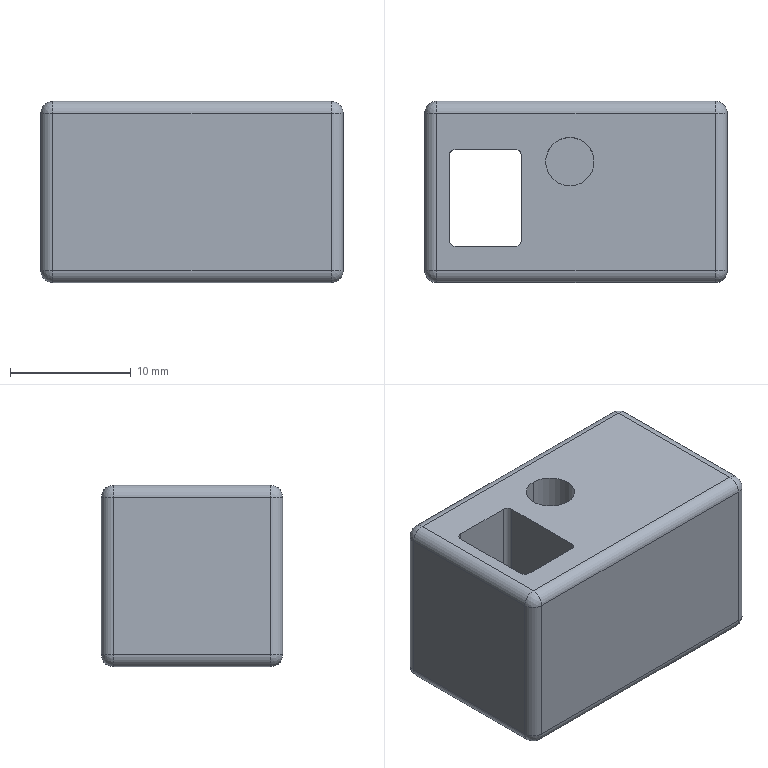NC program | NX | posted with a generic post | part box 25 x 15 x 15 mm
Whole program:
N10 G17 G21 G94 G90
(FLOOR_WALL_COPY , TOOL : D63)
N12 T01 M6
N14 G54
N16 G17 G0 G90 X-47. Y0. S6500 M3
N18 G43 Z30. H1
N20 Z7.
N22 G94 G1 Z4. F1250.
N24 X-44.
N26 X44.
N28 X47.
N30 Z7.
N32 G0 Z30.
N34 X-47.
N36 Z6.
N38 G1 Z3.
N40 X-44.
N42 X44.
N44 X47.
N46 Z6.
N48 G0 Z30.
N50 X-47.
N52 Z5.
N54 G1 Z2.
N56 X-44.
N58 X44.
N60 X47.
N62 Z5.
N64 G0 Z30.
N66 X-47.
N68 Z4.
N70 G1 Z1.
N72 X-44.
N74 X44.
N76 X47.
N78 Z4.
N80 G0 Z30.
N82 X-47.
N84 Z3.
N86 G1 Z0.
N88 X-44.
N90 X44.
N92 X47.
N94 Z3.
N96 G0 Z30.
N98 M5
N100 M2